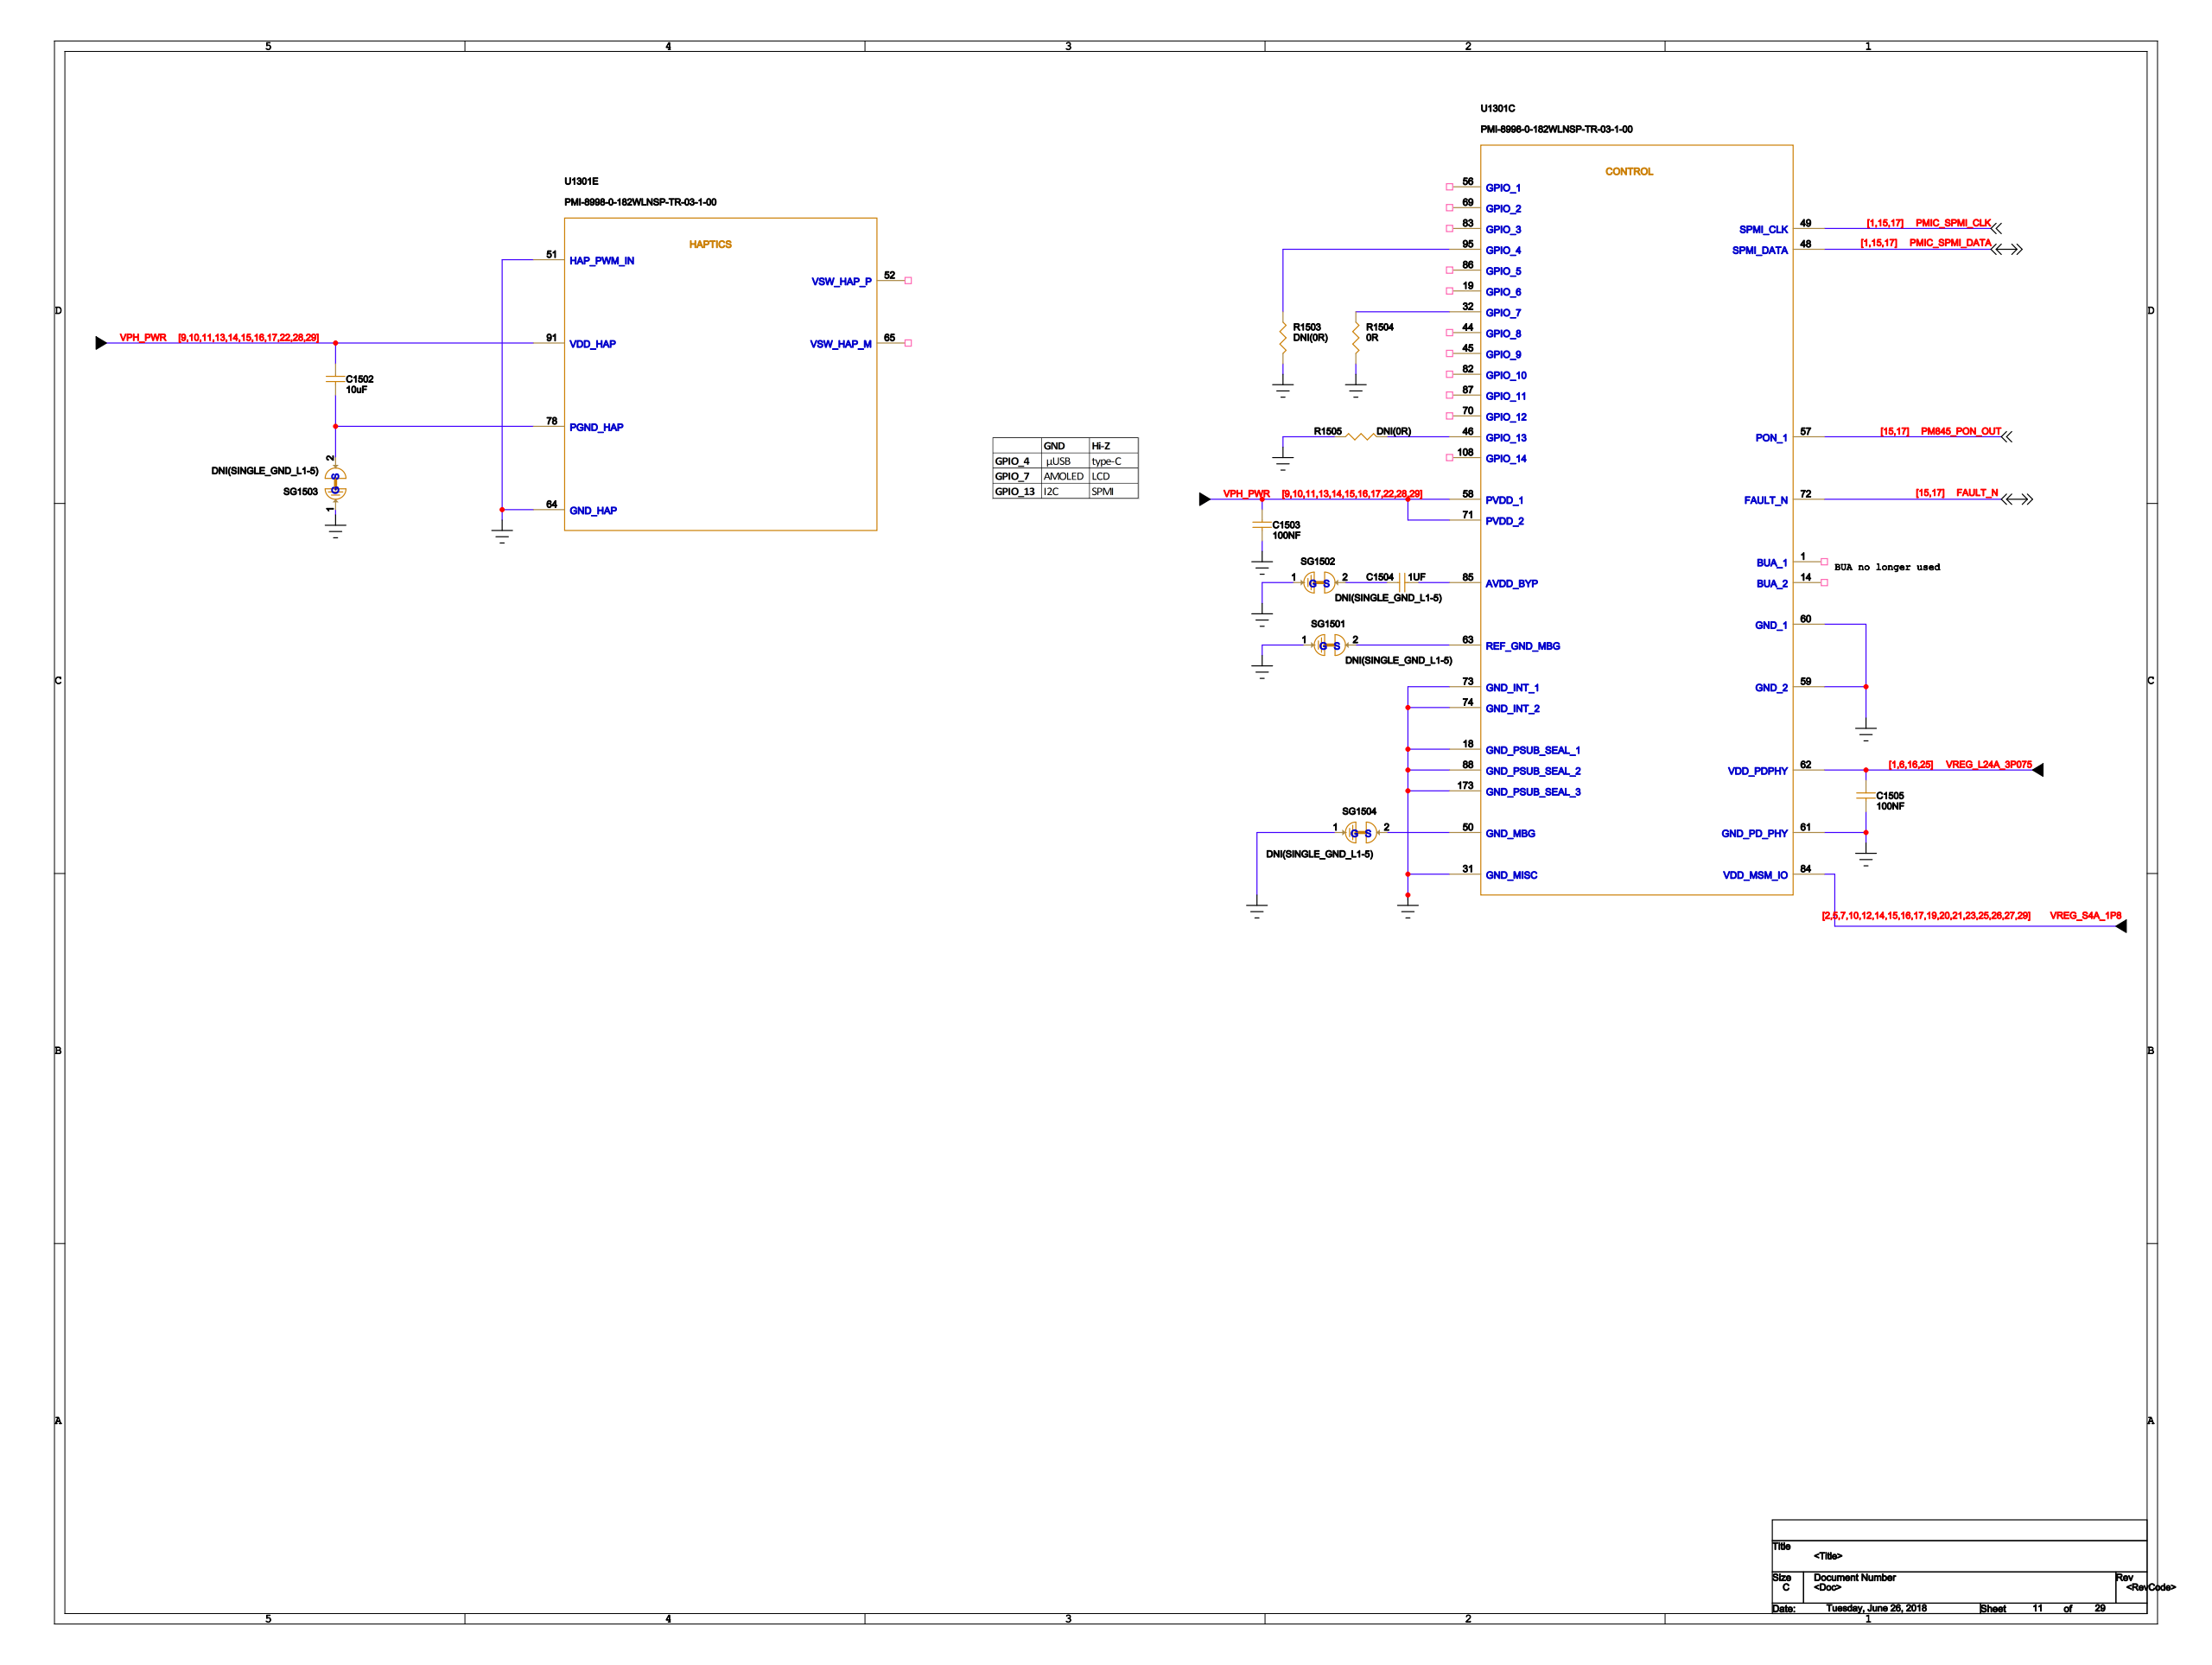Circuit board | Cadence Allegro | 802 parts | 566 nets | one sheet of the schematic
Parts on this sheet (reference | value | footprint):
C1502 | 10uF | 0402-BIG
C1503 | 100NF | C0201
C1504 | 1uF | C0201
C1505 | 100NF | C0201
R1503 | DNI(0R) | R0201
R1504 | 0R | R0201
R1505 | DNI(0R) | R0201
SG1501 | DNI(SINGLE_GND_L1-5) | GND_L1-5
SG1502 | DNI(SINGLE_GND_L1-5) | GND_L1-5
SG1503 | DNI(SINGLE_GND_L1-5) | GND_L1-5
SG1504 | DNI(SINGLE_GND_L1-5) | GND_L1-5
U1301 | PMI-8998-0-182WLNSP-TR-03-1-00 | PMI8998
Nets of these parts (net: part-pin ...):
GND: C1503-2 C1505-2 R1503-2 R1504-2 R1505-1 SG1501-1 SG1502-1 SG1503-1 SG1504-1 U1301-3 U1301-4 U1301-6 U1301-15 U1301-18 U1301-27 U1301-31 U1301-51 U1301-59 U1301-60 U1301-61 U1301-64 U1301-73 U1301-74 U1301-88 U1301-173
VREG_L24A_3P075: C1505-1 U1301-62
VPH_PWR: C1502-1 C1503-1 U1301-2 U1301-22 U1301-58 U1301-71 U1301-91
N169106: C1502-2 SG1503-2 U1301-78
VREG_S4A_1P8: U1301-84
N174063: R1504-1 U1301-32
N174067: R1503-1 U1301-95
N174180: R1505-2 U1301-46
N169102: C1504-1 SG1502-2
N172755: C1504-2 U1301-85
N172443: SG1501-2 U1301-63
N168324: SG1504-2 U1301-50
PMIC_SPMI_DATA: U1301-48
PMIC_SPMI_CLK: U1301-49
PM845_PON_OUT: U1301-57
FAULT_N: U1301-72